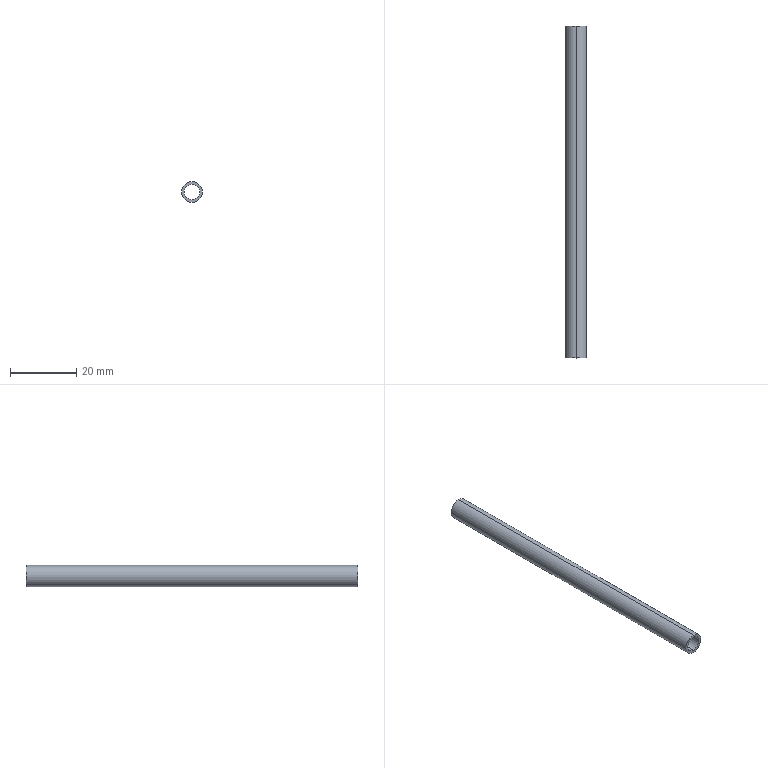Part | STEP file | copper tube 27_default_machined_ | 1 solid | 6 faces | box 6.35 x 100 x 6.35 mm | volume 1395 mm3 | cylinder 4 | plane 2 | commonest cylinder face diameters 4.75 x2 6.35 x2
STEP:
#1=CARTESIAN_POINT('',(0.,0.,0.));
#2=DIRECTION('',(0.,0.,1.));
#3=DIRECTION('',(1.,0.,0.));
#4=AXIS2_PLACEMENT_3D('',#1,#2,#3);
#5=CARTESIAN_POINT('',(0.,100.,-3.175));
#6=VERTEX_POINT('',#5);
#7=CARTESIAN_POINT('',(0.,100.,3.175));
#8=VERTEX_POINT('',#7);
#9=CARTESIAN_POINT('',(0.,100.,0.));
#10=DIRECTION('',(0.,-1.,0.));
#11=DIRECTION('',(0.,0.,-1.));
#12=AXIS2_PLACEMENT_3D('',#9,#10,#11);
#13=CIRCLE('',#12,3.175);
#14=CARTESIAN_POINT('',(0.,100.,0.));
#15=DIRECTION('',(0.,-1.,0.));
#16=DIRECTION('',(0.,0.,-1.));
#17=AXIS2_PLACEMENT_3D('',#14,#15,#16);
#18=CYLINDRICAL_SURFACE('',#17,3.175);
#19=CARTESIAN_POINT('',(0.,0.));
#20=DIRECTION('',(1.,0.));
#21=VECTOR('',#20,1.);
#22=LINE('',#19,#21);
#23=(GEOMETRIC_REPRESENTATION_CONTEXT(2)PARAMETRIC_REPRESENTATION_CONTEXT()REPRESENTATION_CONTEXT('',''));
#24=DEFINITIONAL_REPRESENTATION('',(#22),#23);
#25=PCURVE('',#18,#24);
#26=CARTESIAN_POINT('',(0.,100.,0.));
#27=DIRECTION('',(0.,1.,0.));
#28=DIRECTION('',(0.,0.,1.));
#29=AXIS2_PLACEMENT_3D('',#26,#27,#28);
#30=PLANE('',#29);
#31=CARTESIAN_POINT('',(-3.175,0.));
#32=CARTESIAN_POINT('',(-3.175,5.499));
#33=CARTESIAN_POINT('',(1.587,2.75));
#34=CARTESIAN_POINT('',(6.35,0.));
#35=CARTESIAN_POINT('',(1.587,-2.75));
#36=CARTESIAN_POINT('',(-3.175,-5.499));
#37=CARTESIAN_POINT('',(-3.175,0.));
#38=(BOUNDED_CURVE()B_SPLINE_CURVE(2,(#31,#32,#33,#34,#35,#36,#37),.UNSPECIFIED.,.T.,.F.)B_SPLINE_CURVE_WITH_KNOTS((1,2,2,2,2,1),(-2.094,0.,2.094,4.189,6.283,8.378),.UNSPECIFIED.)CURVE()GEOMETRIC_REPRESENTATION_ITEM()RATIONAL_B_SPLINE_CURVE((1.,0.5,1.,0.5,1.,0.5,1.))REPRESENTATION_ITEM(''));
#39=(GEOMETRIC_REPRESENTATION_CONTEXT(2)PARAMETRIC_REPRESENTATION_CONTEXT()REPRESENTATION_CONTEXT('',''));
#40=DEFINITIONAL_REPRESENTATION('',(#38),#39);
#41=PCURVE('',#30,#40);
#42=SURFACE_CURVE('',#13,(#25,#41),.PCURVE_S1.);
#43=EDGE_CURVE('',#6,#8,#42,.T.);
#44=ORIENTED_EDGE('',*,*,#43,.T.);
#45=CARTESIAN_POINT('',(0.,0.,3.175));
#46=VERTEX_POINT('',#45);
#47=CARTESIAN_POINT('',(0.,100.,3.175));
#48=DIRECTION('',(0.,-1.,0.));
#49=VECTOR('',#48,1.);
#50=LINE('',#47,#49);
#51=CARTESIAN_POINT('',(3.142,0.));
#52=DIRECTION('',(0.,1.));
#53=VECTOR('',#52,1.);
#54=LINE('',#51,#53);
#55=(GEOMETRIC_REPRESENTATION_CONTEXT(2)PARAMETRIC_REPRESENTATION_CONTEXT()REPRESENTATION_CONTEXT('',''));
#56=DEFINITIONAL_REPRESENTATION('',(#54),#55);
#57=PCURVE('',#18,#56);
#58=CARTESIAN_POINT('',(0.,100.,0.));
#59=DIRECTION('',(0.,-1.,0.));
#60=DIRECTION('',(0.,0.,-1.));
#61=AXIS2_PLACEMENT_3D('',#58,#59,#60);
#62=CYLINDRICAL_SURFACE('',#61,3.175);
#63=CARTESIAN_POINT('',(3.142,0.));
#64=DIRECTION('',(0.,1.));
#65=VECTOR('',#64,1.);
#66=LINE('',#63,#65);
#67=(GEOMETRIC_REPRESENTATION_CONTEXT(2)PARAMETRIC_REPRESENTATION_CONTEXT()REPRESENTATION_CONTEXT('',''));
#68=DEFINITIONAL_REPRESENTATION('',(#66),#67);
#69=PCURVE('',#62,#68);
#70=SURFACE_CURVE('',#50,(#57,#69),.PCURVE_S1.);
#71=EDGE_CURVE('',#8,#46,#70,.T.);
#72=ORIENTED_EDGE('',*,*,#71,.T.);
#73=CARTESIAN_POINT('',(0.,0.,-3.175));
#74=VERTEX_POINT('',#73);
#75=CARTESIAN_POINT('',(0.,0.,0.));
#76=DIRECTION('',(0.,1.,0.));
#77=DIRECTION('',(0.,0.,-1.));
#78=AXIS2_PLACEMENT_3D('',#75,#76,#77);
#79=CIRCLE('',#78,3.175);
#80=CARTESIAN_POINT('',(6.283,100.));
#81=DIRECTION('',(-1.,0.));
#82=VECTOR('',#81,1.);
#83=LINE('',#80,#82);
#84=(GEOMETRIC_REPRESENTATION_CONTEXT(2)PARAMETRIC_REPRESENTATION_CONTEXT()REPRESENTATION_CONTEXT('',''));
#85=DEFINITIONAL_REPRESENTATION('',(#83),#84);
#86=PCURVE('',#18,#85);
#87=CARTESIAN_POINT('',(0.,0.,0.));
#88=DIRECTION('',(0.,1.,0.));
#89=DIRECTION('',(0.,0.,1.));
#90=AXIS2_PLACEMENT_3D('',#87,#88,#89);
#91=PLANE('',#90);
#92=CARTESIAN_POINT('',(0.,0.));
#93=DIRECTION('',(-1.,0.));
#94=AXIS2_PLACEMENT_2D('',#92,#93);
#95=CIRCLE('',#94,3.175);
#96=(GEOMETRIC_REPRESENTATION_CONTEXT(2)PARAMETRIC_REPRESENTATION_CONTEXT()REPRESENTATION_CONTEXT('',''));
#97=DEFINITIONAL_REPRESENTATION('',(#95),#96);
#98=PCURVE('',#91,#97);
#99=SURFACE_CURVE('',#79,(#86,#98),.PCURVE_S1.);
#100=EDGE_CURVE('',#46,#74,#99,.T.);
#101=ORIENTED_EDGE('',*,*,#100,.T.);
#102=CARTESIAN_POINT('',(0.,100.,-3.175));
#103=DIRECTION('',(0.,-1.,0.));
#104=VECTOR('',#103,1.);
#105=LINE('',#102,#104);
#106=CARTESIAN_POINT('',(0.,0.));
#107=DIRECTION('',(0.,1.));
#108=VECTOR('',#107,1.);
#109=LINE('',#106,#108);
#110=(GEOMETRIC_REPRESENTATION_CONTEXT(2)PARAMETRIC_REPRESENTATION_CONTEXT()REPRESENTATION_CONTEXT('',''));
#111=DEFINITIONAL_REPRESENTATION('',(#109),#110);
#112=PCURVE('',#18,#111);
#113=CARTESIAN_POINT('',(6.283,0.));
#114=DIRECTION('',(0.,1.));
#115=VECTOR('',#114,1.);
#116=LINE('',#113,#115);
#117=(GEOMETRIC_REPRESENTATION_CONTEXT(2)PARAMETRIC_REPRESENTATION_CONTEXT()REPRESENTATION_CONTEXT('',''));
#118=DEFINITIONAL_REPRESENTATION('',(#116),#117);
#119=PCURVE('',#62,#118);
#120=SURFACE_CURVE('',#105,(#112,#119),.PCURVE_S1.);
#121=EDGE_CURVE('',#6,#74,#120,.T.);
#122=ORIENTED_EDGE('',*,*,#121,.F.);
#123=EDGE_LOOP('',(#44,#72,#101,#122));
#124=FACE_BOUND('',#123,.T.);
#125=ADVANCED_FACE('',(#124),#18,.T.);
#126=CARTESIAN_POINT('',(0.,100.,-2.375));
#127=VERTEX_POINT('',#126);
#128=CARTESIAN_POINT('',(0.,0.,-2.375));
#129=VERTEX_POINT('',#128);
#130=CARTESIAN_POINT('',(0.,100.,-2.375));
#131=DIRECTION('',(0.,-1.,0.));
#132=VECTOR('',#131,1.);
#133=LINE('',#130,#132);
#134=CARTESIAN_POINT('',(0.,100.,0.));
#135=DIRECTION('',(0.,-1.,0.));
#136=DIRECTION('',(0.,0.,-1.));
#137=AXIS2_PLACEMENT_3D('',#134,#135,#136);
#138=CYLINDRICAL_SURFACE('',#137,2.375);
#139=CARTESIAN_POINT('',(6.283,0.));
#140=DIRECTION('',(0.,1.));
#141=VECTOR('',#140,1.);
#142=LINE('',#139,#141);
#143=(GEOMETRIC_REPRESENTATION_CONTEXT(2)PARAMETRIC_REPRESENTATION_CONTEXT()REPRESENTATION_CONTEXT('',''));
#144=DEFINITIONAL_REPRESENTATION('',(#142),#143);
#145=PCURVE('',#138,#144);
#146=CARTESIAN_POINT('',(0.,100.,0.));
#147=DIRECTION('',(0.,-1.,0.));
#148=DIRECTION('',(0.,0.,-1.));
#149=AXIS2_PLACEMENT_3D('',#146,#147,#148);
#150=CYLINDRICAL_SURFACE('',#149,2.375);
#151=CARTESIAN_POINT('',(0.,0.));
#152=DIRECTION('',(0.,1.));
#153=VECTOR('',#152,1.);
#154=LINE('',#151,#153);
#155=(GEOMETRIC_REPRESENTATION_CONTEXT(2)PARAMETRIC_REPRESENTATION_CONTEXT()REPRESENTATION_CONTEXT('',''));
#156=DEFINITIONAL_REPRESENTATION('',(#154),#155);
#157=PCURVE('',#150,#156);
#158=SURFACE_CURVE('',#133,(#145,#157),.PCURVE_S1.);
#159=EDGE_CURVE('',#127,#129,#158,.T.);
#160=ORIENTED_EDGE('',*,*,#159,.T.);
#161=CARTESIAN_POINT('',(0.,0.,2.375));
#162=VERTEX_POINT('',#161);
#163=CARTESIAN_POINT('',(0.,0.,0.));
#164=DIRECTION('',(0.,-1.,0.));
#165=DIRECTION('',(0.,0.,-1.));
#166=AXIS2_PLACEMENT_3D('',#163,#164,#165);
#167=CIRCLE('',#166,2.375);
#168=CARTESIAN_POINT('',(0.,100.));
#169=DIRECTION('',(1.,0.));
#170=VECTOR('',#169,1.);
#171=LINE('',#168,#170);
#172=(GEOMETRIC_REPRESENTATION_CONTEXT(2)PARAMETRIC_REPRESENTATION_CONTEXT()REPRESENTATION_CONTEXT('',''));
#173=DEFINITIONAL_REPRESENTATION('',(#171),#172);
#174=PCURVE('',#138,#173);
#175=CARTESIAN_POINT('',(-2.375,0.));
#176=CARTESIAN_POINT('',(-2.375,4.114));
#177=CARTESIAN_POINT('',(1.188,2.057));
#178=CARTESIAN_POINT('',(4.75,0.));
#179=CARTESIAN_POINT('',(1.188,-2.057));
#180=CARTESIAN_POINT('',(-2.375,-4.114));
#181=CARTESIAN_POINT('',(-2.375,0.));
#182=(BOUNDED_CURVE()B_SPLINE_CURVE(2,(#175,#176,#177,#178,#179,#180,#181),.UNSPECIFIED.,.T.,.F.)B_SPLINE_CURVE_WITH_KNOTS((1,2,2,2,2,1),(-2.094,0.,2.094,4.189,6.283,8.378),.UNSPECIFIED.)CURVE()GEOMETRIC_REPRESENTATION_ITEM()RATIONAL_B_SPLINE_CURVE((1.,0.5,1.,0.5,1.,0.5,1.))REPRESENTATION_ITEM(''));
#183=(GEOMETRIC_REPRESENTATION_CONTEXT(2)PARAMETRIC_REPRESENTATION_CONTEXT()REPRESENTATION_CONTEXT('',''));
#184=DEFINITIONAL_REPRESENTATION('',(#182),#183);
#185=PCURVE('',#91,#184);
#186=SURFACE_CURVE('',#167,(#174,#185),.PCURVE_S1.);
#187=EDGE_CURVE('',#162,#129,#186,.T.);
#188=ORIENTED_EDGE('',*,*,#187,.F.);
#189=CARTESIAN_POINT('',(0.,100.,2.375));
#190=VERTEX_POINT('',#189);
#191=CARTESIAN_POINT('',(0.,100.,2.375));
#192=DIRECTION('',(0.,-1.,0.));
#193=VECTOR('',#192,1.);
#194=LINE('',#191,#193);
#195=CARTESIAN_POINT('',(3.142,0.));
#196=DIRECTION('',(0.,1.));
#197=VECTOR('',#196,1.);
#198=LINE('',#195,#197);
#199=(GEOMETRIC_REPRESENTATION_CONTEXT(2)PARAMETRIC_REPRESENTATION_CONTEXT()REPRESENTATION_CONTEXT('',''));
#200=DEFINITIONAL_REPRESENTATION('',(#198),#199);
#201=PCURVE('',#138,#200);
#202=CARTESIAN_POINT('',(3.142,0.));
#203=DIRECTION('',(0.,1.));
#204=VECTOR('',#203,1.);
#205=LINE('',#202,#204);
#206=(GEOMETRIC_REPRESENTATION_CONTEXT(2)PARAMETRIC_REPRESENTATION_CONTEXT()REPRESENTATION_CONTEXT('',''));
#207=DEFINITIONAL_REPRESENTATION('',(#205),#206);
#208=PCURVE('',#150,#207);
#209=SURFACE_CURVE('',#194,(#201,#208),.PCURVE_S1.);
#210=EDGE_CURVE('',#190,#162,#209,.T.);
#211=ORIENTED_EDGE('',*,*,#210,.F.);
#212=CARTESIAN_POINT('',(0.,100.,0.));
#213=DIRECTION('',(0.,-1.,0.));
#214=DIRECTION('',(0.,0.,-1.));
#215=AXIS2_PLACEMENT_3D('',#212,#213,#214);
#216=CIRCLE('',#215,2.375);
#217=CARTESIAN_POINT('',(0.,0.));
#218=DIRECTION('',(1.,0.));
#219=VECTOR('',#218,1.);
#220=LINE('',#217,#219);
#221=(GEOMETRIC_REPRESENTATION_CONTEXT(2)PARAMETRIC_REPRESENTATION_CONTEXT()REPRESENTATION_CONTEXT('',''));
#222=DEFINITIONAL_REPRESENTATION('',(#220),#221);
#223=PCURVE('',#138,#222);
#224=CARTESIAN_POINT('',(-2.375,0.));
#225=CARTESIAN_POINT('',(-2.375,4.114));
#226=CARTESIAN_POINT('',(1.188,2.057));
#227=CARTESIAN_POINT('',(4.75,0.));
#228=CARTESIAN_POINT('',(1.188,-2.057));
#229=CARTESIAN_POINT('',(-2.375,-4.114));
#230=CARTESIAN_POINT('',(-2.375,0.));
#231=(BOUNDED_CURVE()B_SPLINE_CURVE(2,(#224,#225,#226,#227,#228,#229,#230),.UNSPECIFIED.,.T.,.F.)B_SPLINE_CURVE_WITH_KNOTS((1,2,2,2,2,1),(-2.094,0.,2.094,4.189,6.283,8.378),.UNSPECIFIED.)CURVE()GEOMETRIC_REPRESENTATION_ITEM()RATIONAL_B_SPLINE_CURVE((1.,0.5,1.,0.5,1.,0.5,1.))REPRESENTATION_ITEM(''));
#232=(GEOMETRIC_REPRESENTATION_CONTEXT(2)PARAMETRIC_REPRESENTATION_CONTEXT()REPRESENTATION_CONTEXT('',''));
#233=DEFINITIONAL_REPRESENTATION('',(#231),#232);
#234=PCURVE('',#30,#233);
#235=SURFACE_CURVE('',#216,(#223,#234),.PCURVE_S1.);
#236=EDGE_CURVE('',#190,#127,#235,.T.);
#237=ORIENTED_EDGE('',*,*,#236,.T.);
#238=EDGE_LOOP('',(#160,#188,#211,#237));
#239=FACE_BOUND('',#238,.F.);
#240=ADVANCED_FACE('',(#239),#138,.F.);
#241=ORIENTED_EDGE('',*,*,#71,.F.);
#242=CARTESIAN_POINT('',(0.,100.,0.));
#243=DIRECTION('',(0.,-1.,0.));
#244=DIRECTION('',(0.,0.,-1.));
#245=AXIS2_PLACEMENT_3D('',#242,#243,#244);
#246=CIRCLE('',#245,3.175);
#247=CARTESIAN_POINT('',(0.,0.));
#248=DIRECTION('',(1.,0.));
#249=VECTOR('',#248,1.);
#250=LINE('',#247,#249);
#251=(GEOMETRIC_REPRESENTATION_CONTEXT(2)PARAMETRIC_REPRESENTATION_CONTEXT()REPRESENTATION_CONTEXT('',''));
#252=DEFINITIONAL_REPRESENTATION('',(#250),#251);
#253=PCURVE('',#62,#252);
#254=CARTESIAN_POINT('',(-3.175,0.));
#255=CARTESIAN_POINT('',(-3.175,5.499));
#256=CARTESIAN_POINT('',(1.587,2.75));
#257=CARTESIAN_POINT('',(6.35,0.));
#258=CARTESIAN_POINT('',(1.587,-2.75));
#259=CARTESIAN_POINT('',(-3.175,-5.499));
#260=CARTESIAN_POINT('',(-3.175,0.));
#261=(BOUNDED_CURVE()B_SPLINE_CURVE(2,(#254,#255,#256,#257,#258,#259,#260),.UNSPECIFIED.,.T.,.F.)B_SPLINE_CURVE_WITH_KNOTS((1,2,2,2,2,1),(-2.094,0.,2.094,4.189,6.283,8.378),.UNSPECIFIED.)CURVE()GEOMETRIC_REPRESENTATION_ITEM()RATIONAL_B_SPLINE_CURVE((1.,0.5,1.,0.5,1.,0.5,1.))REPRESENTATION_ITEM(''));
#262=(GEOMETRIC_REPRESENTATION_CONTEXT(2)PARAMETRIC_REPRESENTATION_CONTEXT()REPRESENTATION_CONTEXT('',''));
#263=DEFINITIONAL_REPRESENTATION('',(#261),#262);
#264=PCURVE('',#30,#263);
#265=SURFACE_CURVE('',#246,(#253,#264),.PCURVE_S1.);
#266=EDGE_CURVE('',#8,#6,#265,.T.);
#267=ORIENTED_EDGE('',*,*,#266,.T.);
#268=ORIENTED_EDGE('',*,*,#121,.T.);
#269=CARTESIAN_POINT('',(0.,0.,0.));
#270=DIRECTION('',(0.,1.,0.));
#271=DIRECTION('',(0.,0.,-1.));
#272=AXIS2_PLACEMENT_3D('',#269,#270,#271);
#273=CIRCLE('',#272,3.175);
#274=CARTESIAN_POINT('',(6.283,100.));
#275=DIRECTION('',(-1.,0.));
#276=VECTOR('',#275,1.);
#277=LINE('',#274,#276);
#278=(GEOMETRIC_REPRESENTATION_CONTEXT(2)PARAMETRIC_REPRESENTATION_CONTEXT()REPRESENTATION_CONTEXT('',''));
#279=DEFINITIONAL_REPRESENTATION('',(#277),#278);
#280=PCURVE('',#62,#279);
#281=CARTESIAN_POINT('',(0.,0.));
#282=DIRECTION('',(-1.,0.));
#283=AXIS2_PLACEMENT_2D('',#281,#282);
#284=CIRCLE('',#283,3.175);
#285=(GEOMETRIC_REPRESENTATION_CONTEXT(2)PARAMETRIC_REPRESENTATION_CONTEXT()REPRESENTATION_CONTEXT('',''));
#286=DEFINITIONAL_REPRESENTATION('',(#284),#285);
#287=PCURVE('',#91,#286);
#288=SURFACE_CURVE('',#273,(#280,#287),.PCURVE_S1.);
#289=EDGE_CURVE('',#74,#46,#288,.T.);
#290=ORIENTED_EDGE('',*,*,#289,.T.);
#291=EDGE_LOOP('',(#241,#267,#268,#290));
#292=FACE_BOUND('',#291,.T.);
#293=ADVANCED_FACE('',(#292),#62,.T.);
#294=ORIENTED_EDGE('',*,*,#289,.F.);
#295=ORIENTED_EDGE('',*,*,#100,.F.);
#296=EDGE_LOOP('',(#294,#295));
#297=FACE_BOUND('',#296,.T.);
#298=CARTESIAN_POINT('',(0.,0.,0.));
#299=DIRECTION('',(0.,-1.,0.));
#300=DIRECTION('',(0.,0.,-1.));
#301=AXIS2_PLACEMENT_3D('',#298,#299,#300);
#302=CIRCLE('',#301,2.375);
#303=CARTESIAN_POINT('',(-2.375,0.));
#304=CARTESIAN_POINT('',(-2.375,4.114));
#305=CARTESIAN_POINT('',(1.188,2.057));
#306=CARTESIAN_POINT('',(4.75,0.));
#307=CARTESIAN_POINT('',(1.188,-2.057));
#308=CARTESIAN_POINT('',(-2.375,-4.114));
#309=CARTESIAN_POINT('',(-2.375,0.));
#310=(BOUNDED_CURVE()B_SPLINE_CURVE(2,(#303,#304,#305,#306,#307,#308,#309),.UNSPECIFIED.,.T.,.F.)B_SPLINE_CURVE_WITH_KNOTS((1,2,2,2,2,1),(-2.094,0.,2.094,4.189,6.283,8.378),.UNSPECIFIED.)CURVE()GEOMETRIC_REPRESENTATION_ITEM()RATIONAL_B_SPLINE_CURVE((1.,0.5,1.,0.5,1.,0.5,1.))REPRESENTATION_ITEM(''));
#311=(GEOMETRIC_REPRESENTATION_CONTEXT(2)PARAMETRIC_REPRESENTATION_CONTEXT()REPRESENTATION_CONTEXT('',''));
#312=DEFINITIONAL_REPRESENTATION('',(#310),#311);
#313=PCURVE('',#91,#312);
#314=CARTESIAN_POINT('',(0.,100.));
#315=DIRECTION('',(1.,0.));
#316=VECTOR('',#315,1.);
#317=LINE('',#314,#316);
#318=(GEOMETRIC_REPRESENTATION_CONTEXT(2)PARAMETRIC_REPRESENTATION_CONTEXT()REPRESENTATION_CONTEXT('',''));
#319=DEFINITIONAL_REPRESENTATION('',(#317),#318);
#320=PCURVE('',#150,#319);
#321=SURFACE_CURVE('',#302,(#313,#320),.PCURVE_S1.);
#322=EDGE_CURVE('',#129,#162,#321,.T.);
#323=ORIENTED_EDGE('',*,*,#322,.F.);
#324=ORIENTED_EDGE('',*,*,#187,.F.);
#325=EDGE_LOOP('',(#323,#324));
#326=FACE_BOUND('',#325,.T.);
#327=ADVANCED_FACE('',(#297,#326),#91,.F.);
#328=ORIENTED_EDGE('',*,*,#43,.F.);
#329=ORIENTED_EDGE('',*,*,#266,.F.);
#330=EDGE_LOOP('',(#328,#329));
#331=FACE_BOUND('',#330,.T.);
#332=CARTESIAN_POINT('',(0.,100.,0.));
#333=DIRECTION('',(0.,-1.,0.));
#334=DIRECTION('',(0.,0.,-1.));
#335=AXIS2_PLACEMENT_3D('',#332,#333,#334);
#336=CIRCLE('',#335,2.375);
#337=CARTESIAN_POINT('',(-2.375,0.));
#338=CARTESIAN_POINT('',(-2.375,4.114));
#339=CARTESIAN_POINT('',(1.188,2.057));
#340=CARTESIAN_POINT('',(4.75,0.));
#341=CARTESIAN_POINT('',(1.188,-2.057));
#342=CARTESIAN_POINT('',(-2.375,-4.114));
#343=CARTESIAN_POINT('',(-2.375,0.));
#344=(BOUNDED_CURVE()B_SPLINE_CURVE(2,(#337,#338,#339,#340,#341,#342,#343),.UNSPECIFIED.,.T.,.F.)B_SPLINE_CURVE_WITH_KNOTS((1,2,2,2,2,1),(-2.094,0.,2.094,4.189,6.283,8.378),.UNSPECIFIED.)CURVE()GEOMETRIC_REPRESENTATION_ITEM()RATIONAL_B_SPLINE_CURVE((1.,0.5,1.,0.5,1.,0.5,1.))REPRESENTATION_ITEM(''));
#345=(GEOMETRIC_REPRESENTATION_CONTEXT(2)PARAMETRIC_REPRESENTATION_CONTEXT()REPRESENTATION_CONTEXT('',''));
#346=DEFINITIONAL_REPRESENTATION('',(#344),#345);
#347=PCURVE('',#30,#346);
#348=CARTESIAN_POINT('',(0.,0.));
#349=DIRECTION('',(1.,0.));
#350=VECTOR('',#349,1.);
#351=LINE('',#348,#350);
#352=(GEOMETRIC_REPRESENTATION_CONTEXT(2)PARAMETRIC_REPRESENTATION_CONTEXT()REPRESENTATION_CONTEXT('',''));
#353=DEFINITIONAL_REPRESENTATION('',(#351),#352);
#354=PCURVE('',#150,#353);
#355=SURFACE_CURVE('',#336,(#347,#354),.PCURVE_S1.);
#356=EDGE_CURVE('',#127,#190,#355,.T.);
#357=ORIENTED_EDGE('',*,*,#356,.T.);
#358=ORIENTED_EDGE('',*,*,#236,.T.);
#359=EDGE_LOOP('',(#357,#358));
#360=FACE_BOUND('',#359,.T.);
#361=ADVANCED_FACE('',(#331,#360),#30,.T.);
#362=ORIENTED_EDGE('',*,*,#322,.F.);
#363=ORIENTED_EDGE('',*,*,#159,.F.);
#364=ORIENTED_EDGE('',*,*,#356,.T.);
#365=ORIENTED_EDGE('',*,*,#210,.T.);
#366=EDGE_LOOP('',(#362,#363,#364,#365));
#367=FACE_BOUND('',#366,.F.);
#368=ADVANCED_FACE('',(#367),#150,.F.);
#369=CLOSED_SHELL('',(#125,#240,#293,#327,#361,#368));
#370=MANIFOLD_SOLID_BREP('',#369);
#371=(LENGTH_UNIT()NAMED_UNIT(*)SI_UNIT(.MILLI.,.METRE.));
#372=UNCERTAINTY_MEASURE_WITH_UNIT(LENGTH_MEASURE(0.0000001),#371,'','');
#373=(NAMED_UNIT(*)PLANE_ANGLE_UNIT()SI_UNIT($,.RADIAN.));
#374=(NAMED_UNIT(*)SI_UNIT($,.STERADIAN.)SOLID_ANGLE_UNIT());
#375=(GEOMETRIC_REPRESENTATION_CONTEXT(3)GLOBAL_UNCERTAINTY_ASSIGNED_CONTEXT((#372))GLOBAL_UNIT_ASSIGNED_CONTEXT((#371,#373,#374))REPRESENTATION_CONTEXT('',''));
#376=ADVANCED_BREP_SHAPE_REPRESENTATION('',(#4,#370),#375);